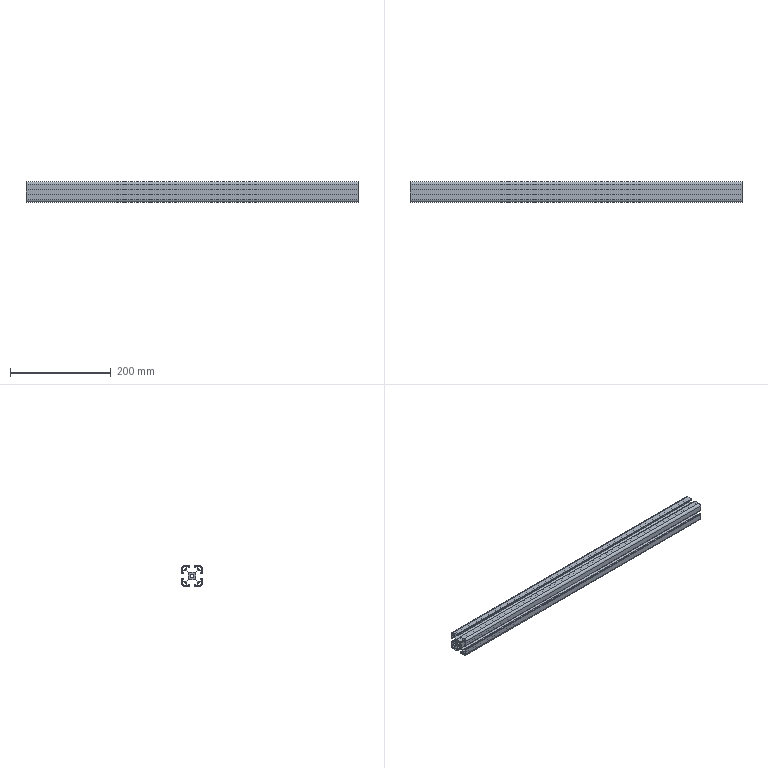Part | 1 solid | 104 faces | box 658 x 40 x 40 mm | volume 379367 mm3 | plane 94 | cylinder 10 | commonest cylinder face diameters 5 x4 9 x4 6.8 x2